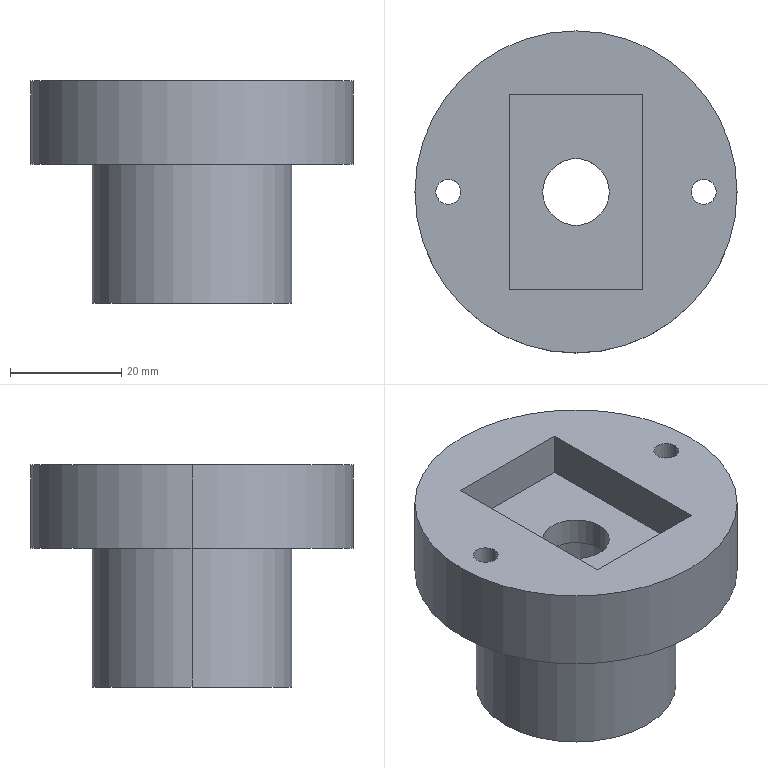Part | SolidWorks | features ICE 3, Extrusion 1, HoleWzd 1 | 1 solid | 27 faces | box 58 x 58 x 40 mm | volume 46736 mm3 | cylinder 16 | plane 11 | commonest cylinder face diameters 4.5 x4 8 x4 12 x2 22 x2 36 x2 58 x2
STEP:
#1=CARTESIAN_POINT('',(-6.,0.,27.));
#2=VERTEX_POINT('',#1);
#3=CARTESIAN_POINT('',(6.,0.,27.));
#4=VERTEX_POINT('',#3);
#5=CARTESIAN_POINT('',(0.,0.,27.));
#6=DIRECTION('',(0.,0.,1.));
#7=DIRECTION('',(1.,0.,0.));
#8=AXIS2_PLACEMENT_3D('',#5,#6,#7);
#9=CIRCLE('',#8,6.);
#10=EDGE_CURVE('',#2,#4,#9,.T.);
#11=ORIENTED_EDGE('',*,*,#10,.F.);
#12=CARTESIAN_POINT('',(-6.,0.,32.));
#13=VERTEX_POINT('',#12);
#14=CARTESIAN_POINT('',(-6.,0.,27.));
#15=DIRECTION('',(0.,0.,1.));
#16=VECTOR('',#15,1000.);
#17=LINE('',#14,#16);
#18=EDGE_CURVE('',#2,#13,#17,.T.);
#19=ORIENTED_EDGE('',*,*,#18,.T.);
#20=CARTESIAN_POINT('',(6.,0.,32.));
#21=VERTEX_POINT('',#20);
#22=CARTESIAN_POINT('',(0.,0.,32.));
#23=DIRECTION('',(0.,0.,1.));
#24=DIRECTION('',(1.,0.,0.));
#25=AXIS2_PLACEMENT_3D('',#22,#23,#24);
#26=CIRCLE('',#25,6.);
#27=EDGE_CURVE('',#13,#21,#26,.T.);
#28=ORIENTED_EDGE('',*,*,#27,.T.);
#29=CARTESIAN_POINT('',(6.,0.,27.));
#30=DIRECTION('',(0.,0.,1.));
#31=VECTOR('',#30,1000.);
#32=LINE('',#29,#31);
#33=EDGE_CURVE('',#4,#21,#32,.T.);
#34=ORIENTED_EDGE('',*,*,#33,.F.);
#35=EDGE_LOOP('',(#11,#19,#28,#34));
#36=FACE_OUTER_BOUND('',#35,.T.);
#37=CARTESIAN_POINT('',(0.,0.,27.));
#38=DIRECTION('',(0.,0.,1.));
#39=DIRECTION('',(1.,0.,0.));
#40=AXIS2_PLACEMENT_3D('',#37,#38,#39);
#41=CYLINDRICAL_SURFACE('',#40,6.);
#42=ADVANCED_FACE('',(#36),#41,.F.);
#43=CARTESIAN_POINT('',(27.,0.,29.6));
#44=VERTEX_POINT('',#43);
#45=CARTESIAN_POINT('',(19.,0.,29.6));
#46=VERTEX_POINT('',#45);
#47=CARTESIAN_POINT('',(23.,0.,29.6));
#48=DIRECTION('',(0.,0.,-1.));
#49=DIRECTION('',(-1.,0.,0.));
#50=AXIS2_PLACEMENT_3D('',#47,#48,#49);
#51=CIRCLE('',#50,4.);
#52=EDGE_CURVE('',#44,#46,#51,.T.);
#53=ORIENTED_EDGE('',*,*,#52,.F.);
#54=CARTESIAN_POINT('',(27.,0.,25.));
#55=VERTEX_POINT('',#54);
#56=CARTESIAN_POINT('',(27.,0.,25.));
#57=DIRECTION('',(0.,0.,-1.));
#58=VECTOR('',#57,1000.);
#59=LINE('',#56,#58);
#60=EDGE_CURVE('',#44,#55,#59,.T.);
#61=ORIENTED_EDGE('',*,*,#60,.T.);
#62=CARTESIAN_POINT('',(19.,0.,25.));
#63=VERTEX_POINT('',#62);
#64=CARTESIAN_POINT('',(23.,0.,25.));
#65=DIRECTION('',(0.,0.,-1.));
#66=DIRECTION('',(-1.,0.,0.));
#67=AXIS2_PLACEMENT_3D('',#64,#65,#66);
#68=CIRCLE('',#67,4.);
#69=EDGE_CURVE('',#55,#63,#68,.T.);
#70=ORIENTED_EDGE('',*,*,#69,.T.);
#71=CARTESIAN_POINT('',(19.,0.,25.));
#72=DIRECTION('',(0.,0.,-1.));
#73=VECTOR('',#72,1000.);
#74=LINE('',#71,#73);
#75=EDGE_CURVE('',#46,#63,#74,.T.);
#76=ORIENTED_EDGE('',*,*,#75,.F.);
#77=EDGE_LOOP('',(#53,#61,#70,#76));
#78=FACE_OUTER_BOUND('',#77,.T.);
#79=CARTESIAN_POINT('',(23.,0.,25.));
#80=DIRECTION('',(0.,0.,-1.));
#81=DIRECTION('',(-1.,0.,0.));
#82=AXIS2_PLACEMENT_3D('',#79,#80,#81);
#83=CYLINDRICAL_SURFACE('',#82,4.);
#84=ADVANCED_FACE('',(#78),#83,.F.);
#85=CARTESIAN_POINT('',(25.25,0.,40.));
#86=VERTEX_POINT('',#85);
#87=CARTESIAN_POINT('',(20.75,0.,40.));
#88=VERTEX_POINT('',#87);
#89=CARTESIAN_POINT('',(23.,0.,40.));
#90=DIRECTION('',(0.,0.,-1.));
#91=DIRECTION('',(-1.,0.,0.));
#92=AXIS2_PLACEMENT_3D('',#89,#90,#91);
#93=CIRCLE('',#92,2.25);
#94=EDGE_CURVE('',#86,#88,#93,.T.);
#95=ORIENTED_EDGE('',*,*,#94,.F.);
#96=CARTESIAN_POINT('',(25.25,0.,29.6));
#97=VERTEX_POINT('',#96);
#98=CARTESIAN_POINT('',(25.25,0.,25.));
#99=DIRECTION('',(0.,0.,-1.));
#100=VECTOR('',#99,1000.);
#101=LINE('',#98,#100);
#102=EDGE_CURVE('',#86,#97,#101,.T.);
#103=ORIENTED_EDGE('',*,*,#102,.T.);
#104=CARTESIAN_POINT('',(20.75,0.,29.6));
#105=VERTEX_POINT('',#104);
#106=CARTESIAN_POINT('',(23.,0.,29.6));
#107=DIRECTION('',(0.,0.,-1.));
#108=DIRECTION('',(-1.,0.,0.));
#109=AXIS2_PLACEMENT_3D('',#106,#107,#108);
#110=CIRCLE('',#109,2.25);
#111=EDGE_CURVE('',#97,#105,#110,.T.);
#112=ORIENTED_EDGE('',*,*,#111,.T.);
#113=CARTESIAN_POINT('',(20.75,0.,25.));
#114=DIRECTION('',(0.,0.,-1.));
#115=VECTOR('',#114,1000.);
#116=LINE('',#113,#115);
#117=EDGE_CURVE('',#88,#105,#116,.T.);
#118=ORIENTED_EDGE('',*,*,#117,.F.);
#119=EDGE_LOOP('',(#95,#103,#112,#118));
#120=FACE_OUTER_BOUND('',#119,.T.);
#121=CARTESIAN_POINT('',(23.,0.,25.));
#122=DIRECTION('',(0.,0.,-1.));
#123=DIRECTION('',(-1.,0.,0.));
#124=AXIS2_PLACEMENT_3D('',#121,#122,#123);
#125=CYLINDRICAL_SURFACE('',#124,2.25);
#126=ADVANCED_FACE('',(#120),#125,.F.);
#127=CARTESIAN_POINT('',(-19.,0.,29.6));
#128=VERTEX_POINT('',#127);
#129=CARTESIAN_POINT('',(-27.,0.,29.6));
#130=VERTEX_POINT('',#129);
#131=CARTESIAN_POINT('',(-23.,0.,29.6));
#132=DIRECTION('',(0.,0.,-1.));
#133=DIRECTION('',(-1.,0.,0.));
#134=AXIS2_PLACEMENT_3D('',#131,#132,#133);
#135=CIRCLE('',#134,4.);
#136=EDGE_CURVE('',#128,#130,#135,.T.);
#137=ORIENTED_EDGE('',*,*,#136,.F.);
#138=CARTESIAN_POINT('',(-19.,0.,25.));
#139=VERTEX_POINT('',#138);
#140=CARTESIAN_POINT('',(-19.,0.,25.));
#141=DIRECTION('',(0.,0.,-1.));
#142=VECTOR('',#141,1000.);
#143=LINE('',#140,#142);
#144=EDGE_CURVE('',#128,#139,#143,.T.);
#145=ORIENTED_EDGE('',*,*,#144,.T.);
#146=CARTESIAN_POINT('',(-27.,0.,25.));
#147=VERTEX_POINT('',#146);
#148=CARTESIAN_POINT('',(-23.,0.,25.));
#149=DIRECTION('',(0.,0.,-1.));
#150=DIRECTION('',(-1.,0.,0.));
#151=AXIS2_PLACEMENT_3D('',#148,#149,#150);
#152=CIRCLE('',#151,4.);
#153=EDGE_CURVE('',#139,#147,#152,.T.);
#154=ORIENTED_EDGE('',*,*,#153,.T.);
#155=CARTESIAN_POINT('',(-27.,0.,25.));
#156=DIRECTION('',(0.,0.,-1.));
#157=VECTOR('',#156,1000.);
#158=LINE('',#155,#157);
#159=EDGE_CURVE('',#130,#147,#158,.T.);
#160=ORIENTED_EDGE('',*,*,#159,.F.);
#161=EDGE_LOOP('',(#137,#145,#154,#160));
#162=FACE_OUTER_BOUND('',#161,.T.);
#163=CARTESIAN_POINT('',(-23.,0.,25.));
#164=DIRECTION('',(0.,0.,-1.));
#165=DIRECTION('',(-1.,0.,0.));
#166=AXIS2_PLACEMENT_3D('',#163,#164,#165);
#167=CYLINDRICAL_SURFACE('',#166,4.);
#168=ADVANCED_FACE('',(#162),#167,.F.);
#169=CARTESIAN_POINT('',(-20.75,0.,40.));
#170=VERTEX_POINT('',#169);
#171=CARTESIAN_POINT('',(-25.25,0.,40.));
#172=VERTEX_POINT('',#171);
#173=CARTESIAN_POINT('',(-23.,0.,40.));
#174=DIRECTION('',(0.,0.,-1.));
#175=DIRECTION('',(-1.,0.,0.));
#176=AXIS2_PLACEMENT_3D('',#173,#174,#175);
#177=CIRCLE('',#176,2.25);
#178=EDGE_CURVE('',#170,#172,#177,.T.);
#179=ORIENTED_EDGE('',*,*,#178,.F.);
#180=CARTESIAN_POINT('',(-20.75,0.,29.6));
#181=VERTEX_POINT('',#180);
#182=CARTESIAN_POINT('',(-20.75,0.,25.));
#183=DIRECTION('',(0.,0.,-1.));
#184=VECTOR('',#183,1000.);
#185=LINE('',#182,#184);
#186=EDGE_CURVE('',#170,#181,#185,.T.);
#187=ORIENTED_EDGE('',*,*,#186,.T.);
#188=CARTESIAN_POINT('',(-25.25,0.,29.6));
#189=VERTEX_POINT('',#188);
#190=CARTESIAN_POINT('',(-23.,0.,29.6));
#191=DIRECTION('',(0.,0.,-1.));
#192=DIRECTION('',(-1.,0.,0.));
#193=AXIS2_PLACEMENT_3D('',#190,#191,#192);
#194=CIRCLE('',#193,2.25);
#195=EDGE_CURVE('',#181,#189,#194,.T.);
#196=ORIENTED_EDGE('',*,*,#195,.T.);
#197=CARTESIAN_POINT('',(-25.25,0.,25.));
#198=DIRECTION('',(0.,0.,-1.));
#199=VECTOR('',#198,1000.);
#200=LINE('',#197,#199);
#201=EDGE_CURVE('',#172,#189,#200,.T.);
#202=ORIENTED_EDGE('',*,*,#201,.F.);
#203=EDGE_LOOP('',(#179,#187,#196,#202));
#204=FACE_OUTER_BOUND('',#203,.T.);
#205=CARTESIAN_POINT('',(-23.,0.,25.));
#206=DIRECTION('',(0.,0.,-1.));
#207=DIRECTION('',(-1.,0.,0.));
#208=AXIS2_PLACEMENT_3D('',#205,#206,#207);
#209=CYLINDRICAL_SURFACE('',#208,2.25);
#210=ADVANCED_FACE('',(#204),#209,.F.);
#211=CARTESIAN_POINT('',(29.,0.,40.));
#212=VERTEX_POINT('',#211);
#213=CARTESIAN_POINT('',(-29.,0.,40.));
#214=VERTEX_POINT('',#213);
#215=CARTESIAN_POINT('',(0.,0.,40.));
#216=DIRECTION('',(0.,0.,1.));
#217=DIRECTION('',(1.,0.,0.));
#218=AXIS2_PLACEMENT_3D('',#215,#216,#217);
#219=CIRCLE('',#218,29.);
#220=EDGE_CURVE('',#212,#214,#219,.T.);
#221=ORIENTED_EDGE('',*,*,#220,.F.);
#222=CARTESIAN_POINT('',(29.,0.,25.));
#223=VERTEX_POINT('',#222);
#224=CARTESIAN_POINT('',(29.,0.,40.));
#225=DIRECTION('',(0.,0.,-1.));
#226=VECTOR('',#225,1000.);
#227=LINE('',#224,#226);
#228=EDGE_CURVE('',#212,#223,#227,.T.);
#229=ORIENTED_EDGE('',*,*,#228,.T.);
#230=CARTESIAN_POINT('',(-29.,0.,25.));
#231=VERTEX_POINT('',#230);
#232=CARTESIAN_POINT('',(0.,0.,25.));
#233=DIRECTION('',(0.,0.,1.));
#234=DIRECTION('',(1.,0.,0.));
#235=AXIS2_PLACEMENT_3D('',#232,#233,#234);
#236=CIRCLE('',#235,29.);
#237=EDGE_CURVE('',#223,#231,#236,.T.);
#238=ORIENTED_EDGE('',*,*,#237,.T.);
#239=CARTESIAN_POINT('',(-29.,0.,40.));
#240=DIRECTION('',(0.,0.,-1.));
#241=VECTOR('',#240,1000.);
#242=LINE('',#239,#241);
#243=EDGE_CURVE('',#214,#231,#242,.T.);
#244=ORIENTED_EDGE('',*,*,#243,.F.);
#245=EDGE_LOOP('',(#221,#229,#238,#244));
#246=FACE_OUTER_BOUND('',#245,.T.);
#247=CARTESIAN_POINT('',(0.,0.,40.));
#248=DIRECTION('',(0.,0.,-1.));
#249=DIRECTION('',(-1.,0.,0.));
#250=AXIS2_PLACEMENT_3D('',#247,#248,#249);
#251=CYLINDRICAL_SURFACE('',#250,29.);
#252=ADVANCED_FACE('',(#246),#251,.T.);
#253=CARTESIAN_POINT('',(18.,0.,25.));
#254=VERTEX_POINT('',#253);
#255=CARTESIAN_POINT('',(-18.,0.,25.));
#256=VERTEX_POINT('',#255);
#257=CARTESIAN_POINT('',(0.,0.,25.));
#258=DIRECTION('',(0.,0.,1.));
#259=DIRECTION('',(1.,0.,0.));
#260=AXIS2_PLACEMENT_3D('',#257,#258,#259);
#261=CIRCLE('',#260,18.);
#262=EDGE_CURVE('',#254,#256,#261,.T.);
#263=ORIENTED_EDGE('',*,*,#262,.F.);
#264=CARTESIAN_POINT('',(18.,0.,0.));
#265=VERTEX_POINT('',#264);
#266=CARTESIAN_POINT('',(18.,0.,25.));
#267=DIRECTION('',(0.,0.,-1.));
#268=VECTOR('',#267,1000.);
#269=LINE('',#266,#268);
#270=EDGE_CURVE('',#254,#265,#269,.T.);
#271=ORIENTED_EDGE('',*,*,#270,.T.);
#272=CARTESIAN_POINT('',(-18.,0.,0.));
#273=VERTEX_POINT('',#272);
#274=CARTESIAN_POINT('',(0.,0.,0.));
#275=DIRECTION('',(0.,0.,1.));
#276=DIRECTION('',(1.,0.,0.));
#277=AXIS2_PLACEMENT_3D('',#274,#275,#276);
#278=CIRCLE('',#277,18.);
#279=EDGE_CURVE('',#265,#273,#278,.T.);
#280=ORIENTED_EDGE('',*,*,#279,.T.);
#281=CARTESIAN_POINT('',(-18.,0.,25.));
#282=DIRECTION('',(0.,0.,-1.));
#283=VECTOR('',#282,1000.);
#284=LINE('',#281,#283);
#285=EDGE_CURVE('',#256,#273,#284,.T.);
#286=ORIENTED_EDGE('',*,*,#285,.F.);
#287=EDGE_LOOP('',(#263,#271,#280,#286));
#288=FACE_OUTER_BOUND('',#287,.T.);
#289=CARTESIAN_POINT('',(0.,0.,25.));
#290=DIRECTION('',(0.,0.,-1.));
#291=DIRECTION('',(-1.,0.,0.));
#292=AXIS2_PLACEMENT_3D('',#289,#290,#291);
#293=CYLINDRICAL_SURFACE('',#292,18.);
#294=ADVANCED_FACE('',(#288),#293,.T.);
#295=CARTESIAN_POINT('',(-11.,0.,27.));
#296=VERTEX_POINT('',#295);
#297=CARTESIAN_POINT('',(11.,0.,27.));
#298=VERTEX_POINT('',#297);
#299=CARTESIAN_POINT('',(0.,0.,27.));
#300=DIRECTION('',(0.,0.,1.));
#301=DIRECTION('',(1.,0.,0.));
#302=AXIS2_PLACEMENT_3D('',#299,#300,#301);
#303=CIRCLE('',#302,11.);
#304=EDGE_CURVE('',#296,#298,#303,.T.);
#305=ORIENTED_EDGE('',*,*,#304,.T.);
#306=CARTESIAN_POINT('',(11.,0.,0.));
#307=VERTEX_POINT('',#306);
#308=CARTESIAN_POINT('',(11.,0.,25.));
#309=DIRECTION('',(0.,0.,-1.));
#310=VECTOR('',#309,1000.);
#311=LINE('',#308,#310);
#312=EDGE_CURVE('',#298,#307,#311,.T.);
#313=ORIENTED_EDGE('',*,*,#312,.T.);
#314=CARTESIAN_POINT('',(-11.,0.,0.));
#315=VERTEX_POINT('',#314);
#316=CARTESIAN_POINT('',(0.,0.,0.));
#317=DIRECTION('',(0.,0.,1.));
#318=DIRECTION('',(1.,0.,0.));
#319=AXIS2_PLACEMENT_3D('',#316,#317,#318);
#320=CIRCLE('',#319,11.);
#321=EDGE_CURVE('',#315,#307,#320,.T.);
#322=ORIENTED_EDGE('',*,*,#321,.F.);
#323=CARTESIAN_POINT('',(-11.,0.,25.));
#324=DIRECTION('',(0.,0.,-1.));
#325=VECTOR('',#324,1000.);
#326=LINE('',#323,#325);
#327=EDGE_CURVE('',#296,#315,#326,.T.);
#328=ORIENTED_EDGE('',*,*,#327,.F.);
#329=EDGE_LOOP('',(#305,#313,#322,#328));
#330=FACE_OUTER_BOUND('',#329,.T.);
#331=CARTESIAN_POINT('',(0.,0.,25.));
#332=DIRECTION('',(0.,0.,-1.));
#333=DIRECTION('',(-1.,0.,0.));
#334=AXIS2_PLACEMENT_3D('',#331,#332,#333);
#335=CYLINDRICAL_SURFACE('',#334,11.);
#336=ADVANCED_FACE('',(#330),#335,.F.);
#337=ORIENTED_EDGE('',*,*,#312,.F.);
#338=CARTESIAN_POINT('',(0.,0.,27.));
#339=DIRECTION('',(0.,0.,1.));
#340=DIRECTION('',(1.,0.,0.));
#341=AXIS2_PLACEMENT_3D('',#338,#339,#340);
#342=CIRCLE('',#341,11.);
#343=EDGE_CURVE('',#298,#296,#342,.T.);
#344=ORIENTED_EDGE('',*,*,#343,.T.);
#345=ORIENTED_EDGE('',*,*,#327,.T.);
#346=CARTESIAN_POINT('',(0.,0.,0.));
#347=DIRECTION('',(0.,0.,1.));
#348=DIRECTION('',(1.,0.,0.));
#349=AXIS2_PLACEMENT_3D('',#346,#347,#348);
#350=CIRCLE('',#349,11.);
#351=EDGE_CURVE('',#307,#315,#350,.T.);
#352=ORIENTED_EDGE('',*,*,#351,.F.);
#353=EDGE_LOOP('',(#337,#344,#345,#352));
#354=FACE_OUTER_BOUND('',#353,.T.);
#355=CARTESIAN_POINT('',(0.,0.,25.));
#356=DIRECTION('',(0.,0.,-1.));
#357=DIRECTION('',(-1.,0.,0.));
#358=AXIS2_PLACEMENT_3D('',#355,#356,#357);
#359=CYLINDRICAL_SURFACE('',#358,11.);
#360=ADVANCED_FACE('',(#354),#359,.F.);
#361=CARTESIAN_POINT('',(0.,0.,0.));
#362=DIRECTION('',(0.,0.,1.));
#363=DIRECTION('',(1.,0.,0.));
#364=AXIS2_PLACEMENT_3D('',#361,#362,#363);
#365=CIRCLE('',#364,18.);
#366=EDGE_CURVE('',#273,#265,#365,.T.);
#367=ORIENTED_EDGE('',*,*,#366,.F.);
#368=ORIENTED_EDGE('',*,*,#279,.F.);
#369=EDGE_LOOP('',(#367,#368));
#370=FACE_OUTER_BOUND('',#369,.T.);
#371=ORIENTED_EDGE('',*,*,#321,.T.);
#372=ORIENTED_EDGE('',*,*,#351,.T.);
#373=EDGE_LOOP('',(#371,#372));
#374=FACE_BOUND('',#373,.T.);
#375=CARTESIAN_POINT('',(0.,0.,0.));
#376=DIRECTION('',(0.,0.,1.));
#377=DIRECTION('',(1.,0.,0.));
#378=AXIS2_PLACEMENT_3D('',#375,#376,#377);
#379=PLANE('',#378);
#380=ADVANCED_FACE('',(#370,#374),#379,.F.);
#381=ORIENTED_EDGE('',*,*,#270,.F.);
#382=CARTESIAN_POINT('',(0.,0.,25.));
#383=DIRECTION('',(0.,0.,1.));
#384=DIRECTION('',(1.,0.,0.));
#385=AXIS2_PLACEMENT_3D('',#382,#383,#384);
#386=CIRCLE('',#385,18.);
#387=EDGE_CURVE('',#256,#254,#386,.T.);
#388=ORIENTED_EDGE('',*,*,#387,.F.);
#389=ORIENTED_EDGE('',*,*,#285,.T.);
#390=ORIENTED_EDGE('',*,*,#366,.T.);
#391=EDGE_LOOP('',(#381,#388,#389,#390));
#392=FACE_OUTER_BOUND('',#391,.T.);
#393=CARTESIAN_POINT('',(0.,0.,25.));
#394=DIRECTION('',(0.,0.,-1.));
#395=DIRECTION('',(-1.,0.,0.));
#396=AXIS2_PLACEMENT_3D('',#393,#394,#395);
#397=CYLINDRICAL_SURFACE('',#396,18.);
#398=ADVANCED_FACE('',(#392),#397,.T.);
#399=CARTESIAN_POINT('',(23.,0.,25.));
#400=DIRECTION('',(0.,0.,-1.));
#401=DIRECTION('',(-1.,0.,0.));
#402=AXIS2_PLACEMENT_3D('',#399,#400,#401);
#403=CIRCLE('',#402,4.);
#404=EDGE_CURVE('',#63,#55,#403,.T.);
#405=ORIENTED_EDGE('',*,*,#404,.F.);
#406=ORIENTED_EDGE('',*,*,#69,.F.);
#407=EDGE_LOOP('',(#405,#406));
#408=FACE_BOUND('',#407,.T.);
#409=CARTESIAN_POINT('',(-23.,0.,25.));
#410=DIRECTION('',(0.,0.,-1.));
#411=DIRECTION('',(-1.,0.,0.));
#412=AXIS2_PLACEMENT_3D('',#409,#410,#411);
#413=CIRCLE('',#412,4.);
#414=EDGE_CURVE('',#147,#139,#413,.T.);
#415=ORIENTED_EDGE('',*,*,#414,.F.);
#416=ORIENTED_EDGE('',*,*,#153,.F.);
#417=EDGE_LOOP('',(#415,#416));
#418=FACE_BOUND('',#417,.T.);
#419=CARTESIAN_POINT('',(0.,0.,25.));
#420=DIRECTION('',(0.,0.,1.));
#421=DIRECTION('',(1.,0.,0.));
#422=AXIS2_PLACEMENT_3D('',#419,#420,#421);
#423=CIRCLE('',#422,29.);
#424=EDGE_CURVE('',#231,#223,#423,.T.);
#425=ORIENTED_EDGE('',*,*,#424,.F.);
#426=ORIENTED_EDGE('',*,*,#237,.F.);
#427=EDGE_LOOP('',(#425,#426));
#428=FACE_OUTER_BOUND('',#427,.T.);
#429=ORIENTED_EDGE('',*,*,#387,.T.);
#430=ORIENTED_EDGE('',*,*,#262,.T.);
#431=EDGE_LOOP('',(#429,#430));
#432=FACE_BOUND('',#431,.T.);
#433=CARTESIAN_POINT('',(0.,0.,25.));
#434=DIRECTION('',(0.,0.,1.));
#435=DIRECTION('',(1.,0.,0.));
#436=AXIS2_PLACEMENT_3D('',#433,#434,#435);
#437=PLANE('',#436);
#438=ADVANCED_FACE('',(#408,#418,#428,#432),#437,.F.);
#439=CARTESIAN_POINT('',(12.,-17.5,40.));
#440=VERTEX_POINT('',#439);
#441=CARTESIAN_POINT('',(12.,17.5,40.));
#442=VERTEX_POINT('',#441);
#443=CARTESIAN_POINT('',(12.,17.5,40.));
#444=DIRECTION('',(0.,1.,0.));
#445=VECTOR('',#444,1000.);
#446=LINE('',#443,#445);
#447=EDGE_CURVE('',#440,#442,#446,.T.);
#448=ORIENTED_EDGE('',*,*,#447,.F.);
#449=CARTESIAN_POINT('',(-12.,-17.5,40.));
#450=VERTEX_POINT('',#449);
#451=CARTESIAN_POINT('',(-12.,-17.5,40.));
#452=DIRECTION('',(1.,0.,0.));
#453=VECTOR('',#452,1000.);
#454=LINE('',#451,#453);
#455=EDGE_CURVE('',#450,#440,#454,.T.);
#456=ORIENTED_EDGE('',*,*,#455,.F.);
#457=CARTESIAN_POINT('',(-12.,17.5,40.));
#458=VERTEX_POINT('',#457);
#459=CARTESIAN_POINT('',(-12.,17.5,40.));
#460=DIRECTION('',(0.,-1.,0.));
#461=VECTOR('',#460,1000.);
#462=LINE('',#459,#461);
#463=EDGE_CURVE('',#458,#450,#462,.T.);
#464=ORIENTED_EDGE('',*,*,#463,.F.);
#465=CARTESIAN_POINT('',(-12.,17.5,40.));
#466=DIRECTION('',(-1.,0.,0.));
#467=VECTOR('',#466,1000.);
#468=LINE('',#465,#467);
#469=EDGE_CURVE('',#442,#458,#468,.T.);
#470=ORIENTED_EDGE('',*,*,#469,.F.);
#471=EDGE_LOOP('',(#448,#456,#464,#470));
#472=FACE_BOUND('',#471,.T.);
#473=CARTESIAN_POINT('',(23.,0.,40.));
#474=DIRECTION('',(0.,0.,-1.));
#475=DIRECTION('',(-1.,0.,0.));
#476=AXIS2_PLACEMENT_3D('',#473,#474,#475);
#477=CIRCLE('',#476,2.25);
#478=EDGE_CURVE('',#88,#86,#477,.T.);
#479=ORIENTED_EDGE('',*,*,#478,.T.);
#480=ORIENTED_EDGE('',*,*,#94,.T.);
#481=EDGE_LOOP('',(#479,#480));
#482=FACE_BOUND('',#481,.T.);
#483=CARTESIAN_POINT('',(-23.,0.,40.));
#484=DIRECTION('',(0.,0.,-1.));
#485=DIRECTION('',(-1.,0.,0.));
#486=AXIS2_PLACEMENT_3D('',#483,#484,#485);
#487=CIRCLE('',#486,2.25);
#488=EDGE_CURVE('',#172,#170,#487,.T.);
#489=ORIENTED_EDGE('',*,*,#488,.T.);
#490=ORIENTED_EDGE('',*,*,#178,.T.);
#491=EDGE_LOOP('',(#489,#490));
#492=FACE_BOUND('',#491,.T.);
#493=CARTESIAN_POINT('',(0.,0.,40.));
#494=DIRECTION('',(0.,0.,1.));
#495=DIRECTION('',(1.,0.,0.));
#496=AXIS2_PLACEMENT_3D('',#493,#494,#495);
#497=CIRCLE('',#496,29.);
#498=EDGE_CURVE('',#214,#212,#497,.T.);
#499=ORIENTED_EDGE('',*,*,#498,.T.);
#500=ORIENTED_EDGE('',*,*,#220,.T.);
#501=EDGE_LOOP('',(#499,#500));
#502=FACE_OUTER_BOUND('',#501,.T.);
#503=CARTESIAN_POINT('',(0.,0.,40.));
#504=DIRECTION('',(0.,0.,1.));
#505=DIRECTION('',(1.,0.,0.));
#506=AXIS2_PLACEMENT_3D('',#503,#504,#505);
#507=PLANE('',#506);
#508=ADVANCED_FACE('',(#472,#482,#492,#502),#507,.T.);
#509=ORIENTED_EDGE('',*,*,#228,.F.);
#510=ORIENTED_EDGE('',*,*,#498,.F.);
#511=ORIENTED_EDGE('',*,*,#243,.T.);
#512=ORIENTED_EDGE('',*,*,#424,.T.);
#513=EDGE_LOOP('',(#509,#510,#511,#512));
#514=FACE_OUTER_BOUND('',#513,.T.);
#515=CARTESIAN_POINT('',(0.,0.,40.));
#516=DIRECTION('',(0.,0.,-1.));
#517=DIRECTION('',(-1.,0.,0.));
#518=AXIS2_PLACEMENT_3D('',#515,#516,#517);
#519=CYLINDRICAL_SURFACE('',#518,29.);
#520=ADVANCED_FACE('',(#514),#519,.T.);
#521=ORIENTED_EDGE('',*,*,#186,.F.);
#522=ORIENTED_EDGE('',*,*,#488,.F.);
#523=ORIENTED_EDGE('',*,*,#201,.T.);
#524=CARTESIAN_POINT('',(-23.,0.,29.6));
#525=DIRECTION('',(0.,0.,-1.));
#526=DIRECTION('',(-1.,0.,0.));
#527=AXIS2_PLACEMENT_3D('',#524,#525,#526);
#528=CIRCLE('',#527,2.25);
#529=EDGE_CURVE('',#189,#181,#528,.T.);
#530=ORIENTED_EDGE('',*,*,#529,.T.);
#531=EDGE_LOOP('',(#521,#522,#523,#530));
#532=FACE_OUTER_BOUND('',#531,.T.);
#533=CARTESIAN_POINT('',(-23.,0.,25.));
#534=DIRECTION('',(0.,0.,-1.));
#535=DIRECTION('',(-1.,0.,0.));
#536=AXIS2_PLACEMENT_3D('',#533,#534,#535);
#537=CYLINDRICAL_SURFACE('',#536,2.25);
#538=ADVANCED_FACE('',(#532),#537,.F.);
#539=ORIENTED_EDGE('',*,*,#529,.F.);
#540=ORIENTED_EDGE('',*,*,#195,.F.);
#541=EDGE_LOOP('',(#539,#540));
#542=FACE_BOUND('',#541,.T.);
#543=CARTESIAN_POINT('',(-23.,0.,29.6));
#544=DIRECTION('',(0.,0.,-1.));
#545=DIRECTION('',(-1.,0.,0.));
#546=AXIS2_PLACEMENT_3D('',#543,#544,#545);
#547=CIRCLE('',#546,4.);
#548=EDGE_CURVE('',#130,#128,#547,.T.);
#549=ORIENTED_EDGE('',*,*,#548,.T.);
#550=ORIENTED_EDGE('',*,*,#136,.T.);
#551=EDGE_LOOP('',(#549,#550));
#552=FACE_OUTER_BOUND('',#551,.T.);
#553=CARTESIAN_POINT('',(-20.75,0.,29.6));
#554=DIRECTION('',(0.,0.,1.));
#555=DIRECTION('',(1.,0.,0.));
#556=AXIS2_PLACEMENT_3D('',#553,#554,#555);
#557=PLANE('',#556);
#558=ADVANCED_FACE('',(#542,#552),#557,.F.);
#559=ORIENTED_EDGE('',*,*,#144,.F.);
#560=ORIENTED_EDGE('',*,*,#548,.F.);
#561=ORIENTED_EDGE('',*,*,#159,.T.);
#562=ORIENTED_EDGE('',*,*,#414,.T.);
#563=EDGE_LOOP('',(#559,#560,#561,#562));
#564=FACE_OUTER_BOUND('',#563,.T.);
#565=CARTESIAN_POINT('',(-23.,0.,25.));
#566=DIRECTION('',(0.,0.,-1.));
#567=DIRECTION('',(-1.,0.,0.));
#568=AXIS2_PLACEMENT_3D('',#565,#566,#567);
#569=CYLINDRICAL_SURFACE('',#568,4.);
#570=ADVANCED_FACE('',(#564),#569,.F.);
#571=ORIENTED_EDGE('',*,*,#102,.F.);
#572=ORIENTED_EDGE('',*,*,#478,.F.);
#573=ORIENTED_EDGE('',*,*,#117,.T.);
#574=CARTESIAN_POINT('',(23.,0.,29.6));
#575=DIRECTION('',(0.,0.,-1.));
#576=DIRECTION('',(-1.,0.,0.));
#577=AXIS2_PLACEMENT_3D('',#574,#575,#576);
#578=CIRCLE('',#577,2.25);
#579=EDGE_CURVE('',#105,#97,#578,.T.);
#580=ORIENTED_EDGE('',*,*,#579,.T.);
#581=EDGE_LOOP('',(#571,#572,#573,#580));
#582=FACE_OUTER_BOUND('',#581,.T.);
#583=CARTESIAN_POINT('',(23.,0.,25.));
#584=DIRECTION('',(0.,0.,-1.));
#585=DIRECTION('',(-1.,0.,0.));
#586=AXIS2_PLACEMENT_3D('',#583,#584,#585);
#587=CYLINDRICAL_SURFACE('',#586,2.25);
#588=ADVANCED_FACE('',(#582),#587,.F.);
#589=ORIENTED_EDGE('',*,*,#579,.F.);
#590=ORIENTED_EDGE('',*,*,#111,.F.);
#591=EDGE_LOOP('',(#589,#590));
#592=FACE_BOUND('',#591,.T.);
#593=CARTESIAN_POINT('',(23.,0.,29.6));
#594=DIRECTION('',(0.,0.,-1.));
#595=DIRECTION('',(-1.,0.,0.));
#596=AXIS2_PLACEMENT_3D('',#593,#594,#595);
#597=CIRCLE('',#596,4.);
#598=EDGE_CURVE('',#46,#44,#597,.T.);
#599=ORIENTED_EDGE('',*,*,#598,.T.);
#600=ORIENTED_EDGE('',*,*,#52,.T.);
#601=EDGE_LOOP('',(#599,#600));
#602=FACE_OUTER_BOUND('',#601,.T.);
#603=CARTESIAN_POINT('',(25.25,0.,29.6));
#604=DIRECTION('',(0.,0.,1.));
#605=DIRECTION('',(1.,0.,0.));
#606=AXIS2_PLACEMENT_3D('',#603,#604,#605);
#607=PLANE('',#606);
#608=ADVANCED_FACE('',(#592,#602),#607,.F.);
#609=ORIENTED_EDGE('',*,*,#60,.F.);
#610=ORIENTED_EDGE('',*,*,#598,.F.);
#611=ORIENTED_EDGE('',*,*,#75,.T.);
#612=ORIENTED_EDGE('',*,*,#404,.T.);
#613=EDGE_LOOP('',(#609,#610,#611,#612));
#614=FACE_OUTER_BOUND('',#613,.T.);
#615=CARTESIAN_POINT('',(23.,0.,25.));
#616=DIRECTION('',(0.,0.,-1.));
#617=DIRECTION('',(-1.,0.,0.));
#618=AXIS2_PLACEMENT_3D('',#615,#616,#617);
#619=CYLINDRICAL_SURFACE('',#618,4.);
#620=ADVANCED_FACE('',(#614),#619,.F.);
#621=ORIENTED_EDGE('',*,*,#447,.T.);
#622=CARTESIAN_POINT('',(12.,17.5,32.));
#623=VERTEX_POINT('',#622);
#624=CARTESIAN_POINT('',(12.,17.5,32.));
#625=DIRECTION('',(0.,0.,1.));
#626=VECTOR('',#625,1000.);
#627=LINE('',#624,#626);
#628=EDGE_CURVE('',#623,#442,#627,.T.);
#629=ORIENTED_EDGE('',*,*,#628,.F.);
#630=CARTESIAN_POINT('',(12.,-17.5,32.));
#631=VERTEX_POINT('',#630);
#632=CARTESIAN_POINT('',(12.,17.5,32.));
#633=DIRECTION('',(0.,1.,0.));
#634=VECTOR('',#633,1000.);
#635=LINE('',#632,#634);
#636=EDGE_CURVE('',#631,#623,#635,.T.);
#637=ORIENTED_EDGE('',*,*,#636,.F.);
#638=CARTESIAN_POINT('',(12.,-17.5,32.));
#639=DIRECTION('',(0.,0.,1.));
#640=VECTOR('',#639,1000.);
#641=LINE('',#638,#640);
#642=EDGE_CURVE('',#631,#440,#641,.T.);
#643=ORIENTED_EDGE('',*,*,#642,.T.);
#644=EDGE_LOOP('',(#621,#629,#637,#643));
#645=FACE_OUTER_BOUND('',#644,.T.);
#646=CARTESIAN_POINT('',(12.,17.5,32.));
#647=DIRECTION('',(1.,0.,0.));
#648=DIRECTION('',(0.,1.,0.));
#649=AXIS2_PLACEMENT_3D('',#646,#647,#648);
#650=PLANE('',#649);
#651=ADVANCED_FACE('',(#645),#650,.F.);
#652=ORIENTED_EDGE('',*,*,#455,.T.);
#653=ORIENTED_EDGE('',*,*,#642,.F.);
#654=CARTESIAN_POINT('',(-12.,-17.5,32.));
#655=VERTEX_POINT('',#654);
#656=CARTESIAN_POINT('',(-12.,-17.5,32.));
#657=DIRECTION('',(1.,0.,0.));
#658=VECTOR('',#657,1000.);
#659=LINE('',#656,#658);
#660=EDGE_CURVE('',#655,#631,#659,.T.);
#661=ORIENTED_EDGE('',*,*,#660,.F.);
#662=CARTESIAN_POINT('',(-12.,-17.5,32.));
#663=DIRECTION('',(0.,0.,1.));
#664=VECTOR('',#663,1000.);
#665=LINE('',#662,#664);
#666=EDGE_CURVE('',#655,#450,#665,.T.);
#667=ORIENTED_EDGE('',*,*,#666,.T.);
#668=EDGE_LOOP('',(#652,#653,#661,#667));
#669=FACE_OUTER_BOUND('',#668,.T.);
#670=CARTESIAN_POINT('',(-12.,-17.5,32.));
#671=DIRECTION('',(0.,-1.,0.));
#672=DIRECTION('',(0.,0.,-1.));
#673=AXIS2_PLACEMENT_3D('',#670,#671,#672);
#674=PLANE('',#673);
#675=ADVANCED_FACE('',(#669),#674,.F.);
#676=ORIENTED_EDGE('',*,*,#463,.T.);
#677=ORIENTED_EDGE('',*,*,#666,.F.);
#678=CARTESIAN_POINT('',(-12.,17.5,32.));
#679=VERTEX_POINT('',#678);
#680=CARTESIAN_POINT('',(-12.,17.5,32.));
#681=DIRECTION('',(0.,-1.,0.));
#682=VECTOR('',#681,1000.);
#683=LINE('',#680,#682);
#684=EDGE_CURVE('',#679,#655,#683,.T.);
#685=ORIENTED_EDGE('',*,*,#684,.F.);
#686=CARTESIAN_POINT('',(-12.,17.5,32.));
#687=DIRECTION('',(0.,0.,1.));
#688=VECTOR('',#687,1000.);
#689=LINE('',#686,#688);
#690=EDGE_CURVE('',#679,#458,#689,.T.);
#691=ORIENTED_EDGE('',*,*,#690,.T.);
#692=EDGE_LOOP('',(#676,#677,#685,#691));
#693=FACE_OUTER_BOUND('',#692,.T.);
#694=CARTESIAN_POINT('',(-12.,17.5,32.));
#695=DIRECTION('',(-1.,0.,0.));
#696=DIRECTION('',(0.,-1.,0.));
#697=AXIS2_PLACEMENT_3D('',#694,#695,#696);
#698=PLANE('',#697);
#699=ADVANCED_FACE('',(#693),#698,.F.);
#700=ORIENTED_EDGE('',*,*,#469,.T.);
#701=ORIENTED_EDGE('',*,*,#690,.F.);
#702=CARTESIAN_POINT('',(-12.,17.5,32.));
#703=DIRECTION('',(-1.,0.,0.));
#704=VECTOR('',#703,1000.);
#705=LINE('',#702,#704);
#706=EDGE_CURVE('',#623,#679,#705,.T.);
#707=ORIENTED_EDGE('',*,*,#706,.F.);
#708=ORIENTED_EDGE('',*,*,#628,.T.);
#709=EDGE_LOOP('',(#700,#701,#707,#708));
#710=FACE_OUTER_BOUND('',#709,.T.);
#711=CARTESIAN_POINT('',(-12.,17.5,32.));
#712=DIRECTION('',(0.,1.,0.));
#713=DIRECTION('',(0.,0.,1.));
#714=AXIS2_PLACEMENT_3D('',#711,#712,#713);
#715=PLANE('',#714);
#716=ADVANCED_FACE('',(#710),#715,.F.);
#717=ORIENTED_EDGE('',*,*,#636,.T.);
#718=ORIENTED_EDGE('',*,*,#706,.T.);
#719=ORIENTED_EDGE('',*,*,#684,.T.);
#720=ORIENTED_EDGE('',*,*,#660,.T.);
#721=EDGE_LOOP('',(#717,#718,#719,#720));
#722=FACE_OUTER_BOUND('',#721,.T.);
#723=CARTESIAN_POINT('',(0.,0.,32.));
#724=DIRECTION('',(0.,0.,1.));
#725=DIRECTION('',(1.,0.,0.));
#726=AXIS2_PLACEMENT_3D('',#723,#724,#725);
#727=CIRCLE('',#726,6.);
#728=EDGE_CURVE('',#21,#13,#727,.T.);
#729=ORIENTED_EDGE('',*,*,#728,.F.);
#730=ORIENTED_EDGE('',*,*,#27,.F.);
#731=EDGE_LOOP('',(#729,#730));
#732=FACE_BOUND('',#731,.T.);
#733=CARTESIAN_POINT('',(0.,0.,32.));
#734=DIRECTION('',(0.,0.,1.));
#735=DIRECTION('',(1.,0.,0.));
#736=AXIS2_PLACEMENT_3D('',#733,#734,#735);
#737=PLANE('',#736);
#738=ADVANCED_FACE('',(#722,#732),#737,.T.);
#739=CARTESIAN_POINT('',(0.,0.,27.));
#740=DIRECTION('',(0.,0.,1.));
#741=DIRECTION('',(1.,0.,0.));
#742=AXIS2_PLACEMENT_3D('',#739,#740,#741);
#743=CIRCLE('',#742,6.);
#744=EDGE_CURVE('',#4,#2,#743,.T.);
#745=ORIENTED_EDGE('',*,*,#744,.T.);
#746=ORIENTED_EDGE('',*,*,#10,.T.);
#747=EDGE_LOOP('',(#745,#746));
#748=FACE_BOUND('',#747,.T.);
#749=ORIENTED_EDGE('',*,*,#304,.F.);
#750=ORIENTED_EDGE('',*,*,#343,.F.);
#751=EDGE_LOOP('',(#749,#750));
#752=FACE_OUTER_BOUND('',#751,.T.);
#753=CARTESIAN_POINT('',(0.,0.,27.));
#754=DIRECTION('',(0.,0.,1.));
#755=DIRECTION('',(1.,0.,0.));
#756=AXIS2_PLACEMENT_3D('',#753,#754,#755);
#757=PLANE('',#756);
#758=ADVANCED_FACE('',(#748,#752),#757,.F.);
#759=ORIENTED_EDGE('',*,*,#18,.F.);
#760=ORIENTED_EDGE('',*,*,#744,.F.);
#761=ORIENTED_EDGE('',*,*,#33,.T.);
#762=ORIENTED_EDGE('',*,*,#728,.T.);
#763=EDGE_LOOP('',(#759,#760,#761,#762));
#764=FACE_OUTER_BOUND('',#763,.T.);
#765=CARTESIAN_POINT('',(0.,0.,27.));
#766=DIRECTION('',(0.,0.,1.));
#767=DIRECTION('',(1.,0.,0.));
#768=AXIS2_PLACEMENT_3D('',#765,#766,#767);
#769=CYLINDRICAL_SURFACE('',#768,6.);
#770=ADVANCED_FACE('',(#764),#769,.F.);
#771=CLOSED_SHELL('',(#42,#84,#126,#168,#210,#252,#294,#336,#360,#380,#398,#438,#508,#520,#538,#558,#570,#588,#608,#620,#651,#675,#699,#716,#738,#758,#770));
#772=MANIFOLD_SOLID_BREP('',#771);
#773=CARTESIAN_POINT('',(0.,0.,0.));
#774=DIRECTION('',(0.,0.,1.));
#775=DIRECTION('',(1.,0.,0.));
#776=AXIS2_PLACEMENT_3D('',#773,#774,#775);
#777=(LENGTH_UNIT()NAMED_UNIT(*)SI_UNIT(.MILLI.,.METRE.));
#778=UNCERTAINTY_MEASURE_WITH_UNIT(LENGTH_MEASURE(0.00001),#777,'','');
#779=(NAMED_UNIT(*)PLANE_ANGLE_UNIT()SI_UNIT($,.RADIAN.));
#780=(NAMED_UNIT(*)SI_UNIT($,.STERADIAN.)SOLID_ANGLE_UNIT());
#781=(GEOMETRIC_REPRESENTATION_CONTEXT(3)GLOBAL_UNCERTAINTY_ASSIGNED_CONTEXT((#778))GLOBAL_UNIT_ASSIGNED_CONTEXT((#777,#779,#780))REPRESENTATION_CONTEXT('',''));
#782=ADVANCED_BREP_SHAPE_REPRESENTATION('',(#772,#776),#781);